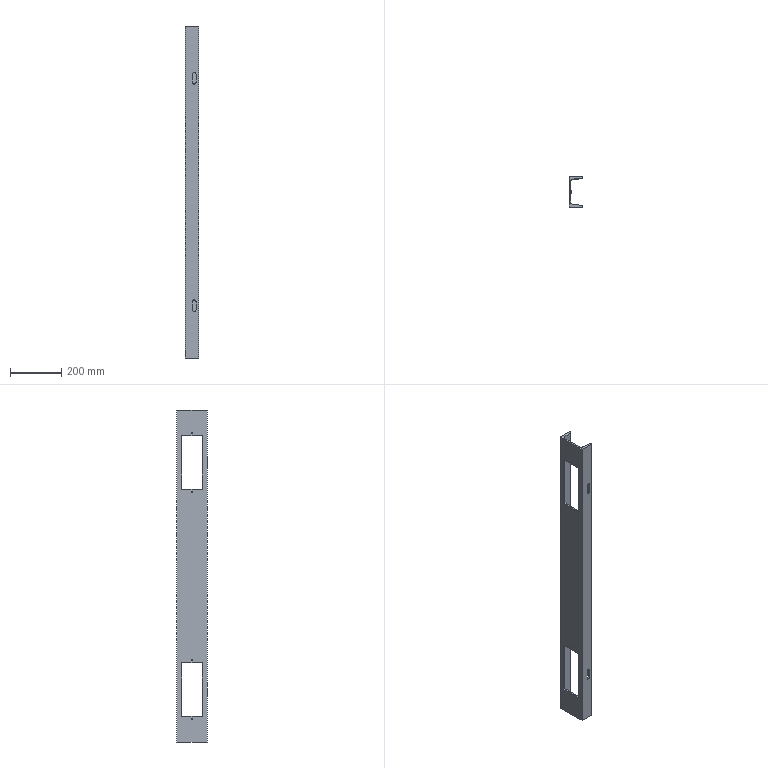Part | SolidWorks | features BaseBody 1 | 1 solid | 78 faces | box 53 x 120 x 1300 mm | volume 1800806 mm3 | plane 54 | cylinder 24 | commonest cylinder face diameters 5 x8 5.5 x8 15 x4 9 x2 18 x2